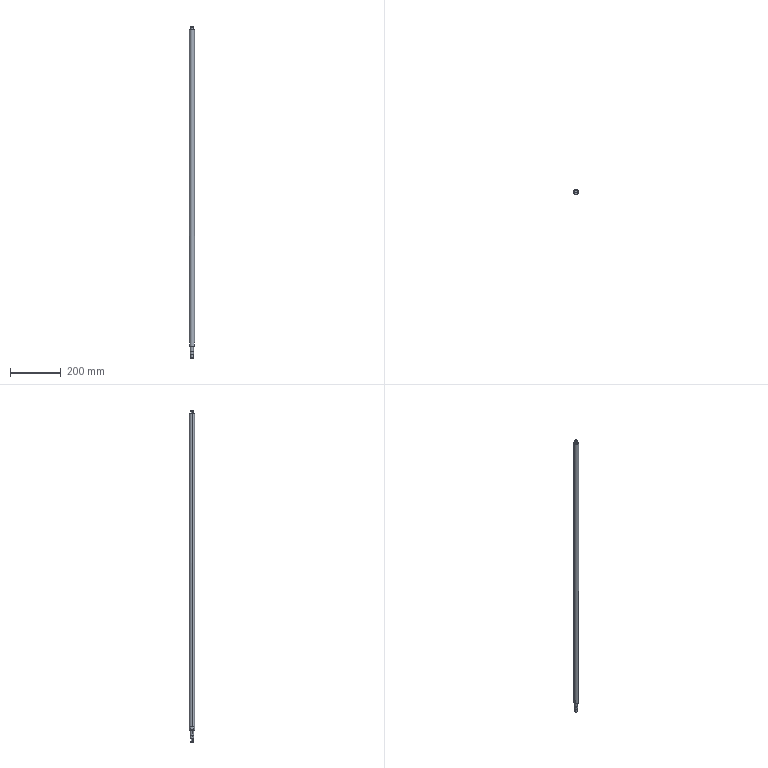Part | STEP file | SM140A-20-1140D-140A-60016 Lead screw | 1 solid | 35 faces | box 20 x 20 x 1305 mm | volume 397382 mm3 | cylinder 16 | plane 15 | cone 4 | commonest cylinder face diameters 10 x6 12 x4 9.6 x2 10.4 x2 20 x2